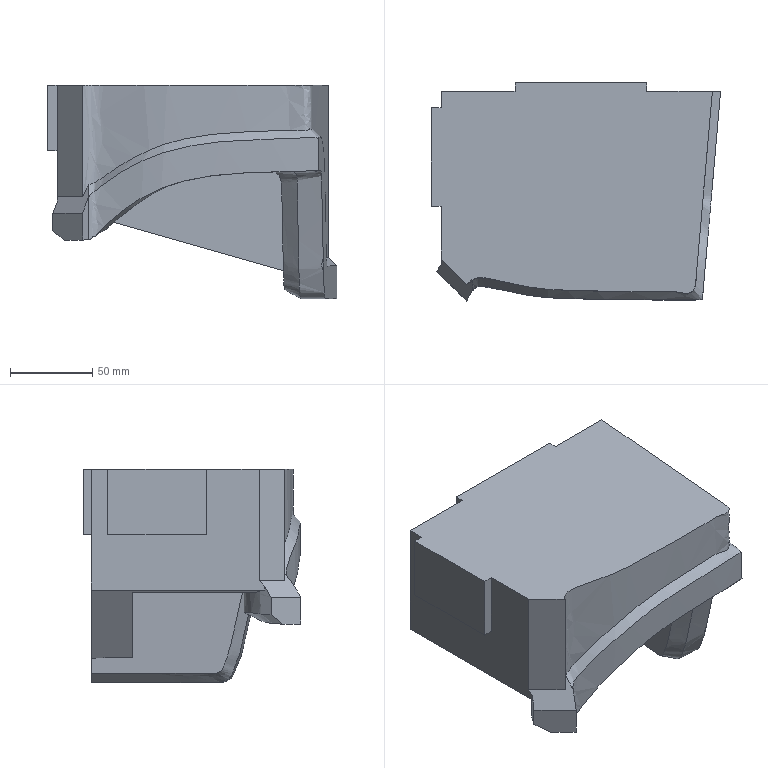Part | NX | features solid 2 | 1 solid | 39 faces | box 176.093 x 132.658 x 130.042 mm | volume 1204341 mm3 | plane 24 | spline 10 | cylinder 5 | commonest cylinder face diameters 30 x5